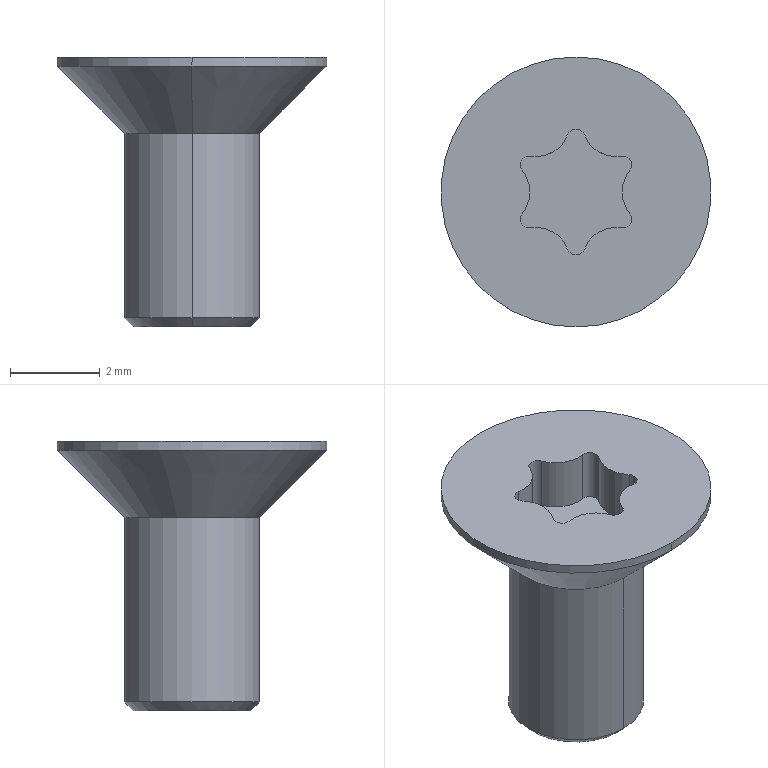Part | STEP file | ASND-0110-0219110027 | 1 solid | 26 faces | box 6 x 6 x 6 mm | volume 55.363 mm3 | cylinder 19 | cone 4 | plane 3 | commonest cylinder face diameters 0.4 x8 1.495 x7 3 x2 6 x2